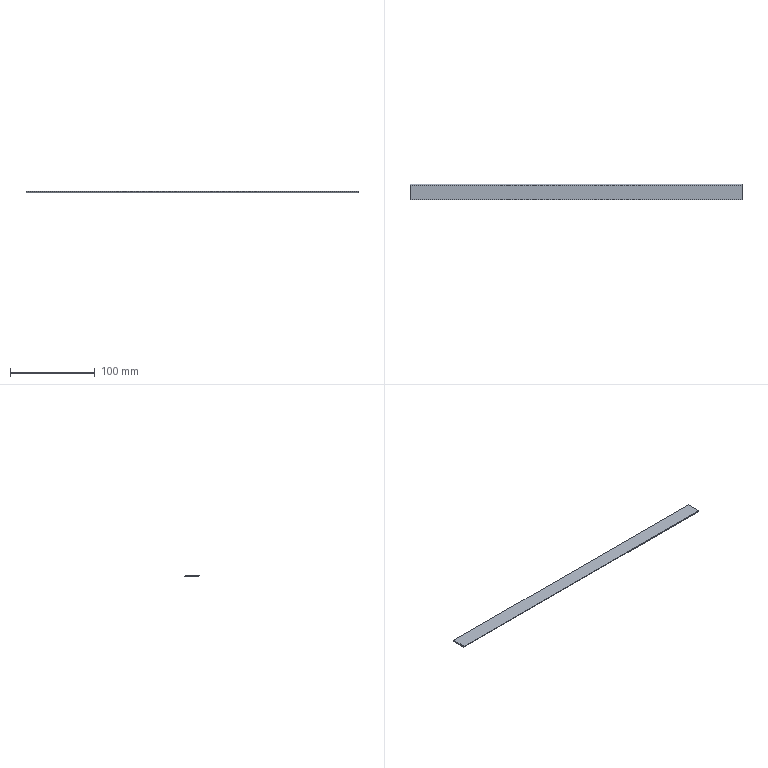Part | SolidWorks | features BaseBody 1 | 1 solid | 6 faces | box 391 x 18.475 x 2 mm | volume 13545 mm3 | plane 6
STEP:
#1=CARTESIAN_POINT('',(195.5,11.012,-2.));
#2=VERTEX_POINT('',#1);
#3=CARTESIAN_POINT('',(-195.5,11.012,-2.));
#4=VERTEX_POINT('',#3);
#5=CARTESIAN_POINT('',(0.,11.012,-2.));
#6=DIRECTION('',(-1.,0.,0.));
#7=VECTOR('',#6,1000.);
#8=LINE('',#5,#7);
#9=EDGE_CURVE('',#2,#4,#8,.T.);
#10=ORIENTED_EDGE('',*,*,#9,.T.);
#11=CARTESIAN_POINT('',(-195.5,9.857,0.));
#12=VERTEX_POINT('',#11);
#13=CARTESIAN_POINT('',(-195.5,13.,-5.443));
#14=DIRECTION('',(0.,-0.5,0.866));
#15=VECTOR('',#14,1000.);
#16=LINE('',#13,#15);
#17=EDGE_CURVE('',#4,#12,#16,.T.);
#18=ORIENTED_EDGE('',*,*,#17,.T.);
#19=CARTESIAN_POINT('',(195.5,9.857,0.));
#20=VERTEX_POINT('',#19);
#21=CARTESIAN_POINT('',(0.,9.857,0.));
#22=DIRECTION('',(-1.,0.,0.));
#23=VECTOR('',#22,1000.);
#24=LINE('',#21,#23);
#25=EDGE_CURVE('',#20,#12,#24,.T.);
#26=ORIENTED_EDGE('',*,*,#25,.F.);
#27=CARTESIAN_POINT('',(195.5,13.,-5.443));
#28=DIRECTION('',(0.,-0.5,0.866));
#29=VECTOR('',#28,1000.);
#30=LINE('',#27,#29);
#31=EDGE_CURVE('',#2,#20,#30,.T.);
#32=ORIENTED_EDGE('',*,*,#31,.F.);
#33=EDGE_LOOP('',(#10,#18,#26,#32));
#34=FACE_OUTER_BOUND('',#33,.T.);
#35=CARTESIAN_POINT('',(195.5,13.,-5.443));
#36=DIRECTION('',(0.,-0.866,-0.5));
#37=DIRECTION('',(0.,0.5,-0.866));
#38=AXIS2_PLACEMENT_3D('',#35,#36,#37);
#39=PLANE('',#38);
#40=ADVANCED_FACE('',(#34),#39,.F.);
#41=CARTESIAN_POINT('',(-195.5,-6.309,-2.));
#42=VERTEX_POINT('',#41);
#43=CARTESIAN_POINT('',(195.5,-6.309,-2.));
#44=VERTEX_POINT('',#43);
#45=CARTESIAN_POINT('',(0.,-6.309,-2.));
#46=DIRECTION('',(1.,0.,0.));
#47=VECTOR('',#46,1000.);
#48=LINE('',#45,#47);
#49=EDGE_CURVE('',#42,#44,#48,.T.);
#50=ORIENTED_EDGE('',*,*,#49,.T.);
#51=CARTESIAN_POINT('',(195.5,-7.463,0.));
#52=VERTEX_POINT('',#51);
#53=CARTESIAN_POINT('',(195.5,-10.24,4.81));
#54=DIRECTION('',(0.,0.5,-0.866));
#55=VECTOR('',#54,1000.);
#56=LINE('',#53,#55);
#57=EDGE_CURVE('',#52,#44,#56,.T.);
#58=ORIENTED_EDGE('',*,*,#57,.F.);
#59=CARTESIAN_POINT('',(-195.5,-7.463,0.));
#60=VERTEX_POINT('',#59);
#61=CARTESIAN_POINT('',(0.,-7.463,0.));
#62=DIRECTION('',(1.,0.,0.));
#63=VECTOR('',#62,1000.);
#64=LINE('',#61,#63);
#65=EDGE_CURVE('',#60,#52,#64,.T.);
#66=ORIENTED_EDGE('',*,*,#65,.F.);
#67=CARTESIAN_POINT('',(-195.5,-10.24,4.81));
#68=DIRECTION('',(0.,0.5,-0.866));
#69=VECTOR('',#68,1000.);
#70=LINE('',#67,#69);
#71=EDGE_CURVE('',#60,#42,#70,.T.);
#72=ORIENTED_EDGE('',*,*,#71,.T.);
#73=EDGE_LOOP('',(#50,#58,#66,#72));
#74=FACE_OUTER_BOUND('',#73,.T.);
#75=CARTESIAN_POINT('',(195.5,-10.24,4.81));
#76=DIRECTION('',(0.,0.866,0.5));
#77=DIRECTION('',(1.,0.,0.));
#78=AXIS2_PLACEMENT_3D('',#75,#76,#77);
#79=PLANE('',#78);
#80=ADVANCED_FACE('',(#74),#79,.F.);
#81=CARTESIAN_POINT('',(195.5,15.,0.));
#82=DIRECTION('',(0.,1.,0.));
#83=VECTOR('',#82,1000.);
#84=LINE('',#81,#83);
#85=EDGE_CURVE('',#52,#20,#84,.T.);
#86=ORIENTED_EDGE('',*,*,#85,.T.);
#87=ORIENTED_EDGE('',*,*,#25,.T.);
#88=CARTESIAN_POINT('',(-195.5,15.,0.));
#89=DIRECTION('',(0.,-1.,0.));
#90=VECTOR('',#89,1000.);
#91=LINE('',#88,#90);
#92=EDGE_CURVE('',#12,#60,#91,.T.);
#93=ORIENTED_EDGE('',*,*,#92,.T.);
#94=ORIENTED_EDGE('',*,*,#65,.T.);
#95=EDGE_LOOP('',(#86,#87,#93,#94));
#96=FACE_OUTER_BOUND('',#95,.T.);
#97=CARTESIAN_POINT('',(0.,0.,0.));
#98=DIRECTION('',(0.,0.,-1.));
#99=DIRECTION('',(0.,-1.,0.));
#100=AXIS2_PLACEMENT_3D('',#97,#98,#99);
#101=PLANE('',#100);
#102=ADVANCED_FACE('',(#96),#101,.F.);
#103=ORIENTED_EDGE('',*,*,#9,.F.);
#104=CARTESIAN_POINT('',(195.5,15.,-2.));
#105=DIRECTION('',(0.,1.,0.));
#106=VECTOR('',#105,1000.);
#107=LINE('',#104,#106);
#108=EDGE_CURVE('',#44,#2,#107,.T.);
#109=ORIENTED_EDGE('',*,*,#108,.F.);
#110=ORIENTED_EDGE('',*,*,#49,.F.);
#111=CARTESIAN_POINT('',(-195.5,15.,-2.));
#112=DIRECTION('',(0.,-1.,0.));
#113=VECTOR('',#112,1000.);
#114=LINE('',#111,#113);
#115=EDGE_CURVE('',#4,#42,#114,.T.);
#116=ORIENTED_EDGE('',*,*,#115,.F.);
#117=EDGE_LOOP('',(#103,#109,#110,#116));
#118=FACE_OUTER_BOUND('',#117,.T.);
#119=CARTESIAN_POINT('',(0.,0.,-2.));
#120=DIRECTION('',(0.,0.,-1.));
#121=DIRECTION('',(0.,-1.,0.));
#122=AXIS2_PLACEMENT_3D('',#119,#120,#121);
#123=PLANE('',#122);
#124=ADVANCED_FACE('',(#118),#123,.T.);
#125=ORIENTED_EDGE('',*,*,#31,.T.);
#126=ORIENTED_EDGE('',*,*,#85,.F.);
#127=ORIENTED_EDGE('',*,*,#57,.T.);
#128=ORIENTED_EDGE('',*,*,#108,.T.);
#129=EDGE_LOOP('',(#125,#126,#127,#128));
#130=FACE_OUTER_BOUND('',#129,.T.);
#131=CARTESIAN_POINT('',(195.5,15.,-2.));
#132=DIRECTION('',(1.,0.,0.));
#133=DIRECTION('',(0.,1.,0.));
#134=AXIS2_PLACEMENT_3D('',#131,#132,#133);
#135=PLANE('',#134);
#136=ADVANCED_FACE('',(#130),#135,.T.);
#137=ORIENTED_EDGE('',*,*,#17,.F.);
#138=ORIENTED_EDGE('',*,*,#115,.T.);
#139=ORIENTED_EDGE('',*,*,#71,.F.);
#140=ORIENTED_EDGE('',*,*,#92,.F.);
#141=EDGE_LOOP('',(#137,#138,#139,#140));
#142=FACE_OUTER_BOUND('',#141,.T.);
#143=CARTESIAN_POINT('',(-195.5,15.,-2.));
#144=DIRECTION('',(-1.,0.,0.));
#145=DIRECTION('',(0.,0.,1.));
#146=AXIS2_PLACEMENT_3D('',#143,#144,#145);
#147=PLANE('',#146);
#148=ADVANCED_FACE('',(#142),#147,.T.);
#149=CLOSED_SHELL('',(#40,#80,#102,#124,#136,#148));
#150=MANIFOLD_SOLID_BREP('',#149);
#151=CARTESIAN_POINT('',(0.,0.,0.));
#152=DIRECTION('',(0.,0.,1.));
#153=DIRECTION('',(1.,0.,0.));
#154=AXIS2_PLACEMENT_3D('',#151,#152,#153);
#155=(LENGTH_UNIT()NAMED_UNIT(*)SI_UNIT(.MILLI.,.METRE.));
#156=UNCERTAINTY_MEASURE_WITH_UNIT(LENGTH_MEASURE(0.00001),#155,'','');
#157=(NAMED_UNIT(*)PLANE_ANGLE_UNIT()SI_UNIT($,.RADIAN.));
#158=(NAMED_UNIT(*)SI_UNIT($,.STERADIAN.)SOLID_ANGLE_UNIT());
#159=(GEOMETRIC_REPRESENTATION_CONTEXT(3)GLOBAL_UNCERTAINTY_ASSIGNED_CONTEXT((#156))GLOBAL_UNIT_ASSIGNED_CONTEXT((#155,#157,#158))REPRESENTATION_CONTEXT('',''));
#160=ADVANCED_BREP_SHAPE_REPRESENTATION('',(#150,#154),#159);